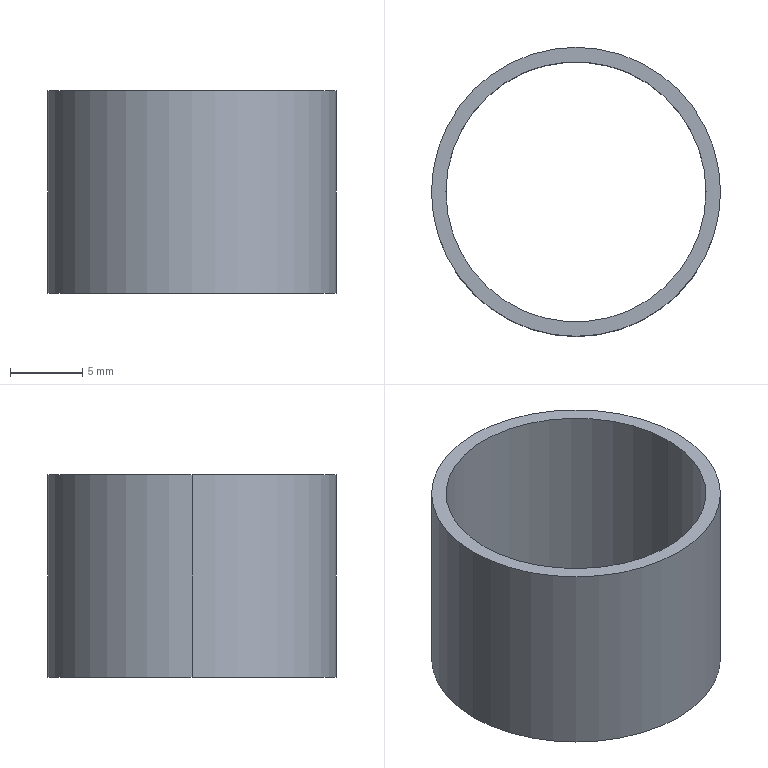Part | STEP file | Oil-Free Bushing JH-B-18-14 | 1 solid | 6 faces | box 20 x 20 x 14 mm | volume 835.664 mm3 | cylinder 4 | plane 2 | commonest cylinder face diameters 18 x2 20 x2
STEP:
#1=CARTESIAN_POINT('',(0.,0.,0.));
#2=DIRECTION('',(0.,0.,1.));
#3=DIRECTION('',(1.,0.,0.));
#4=AXIS2_PLACEMENT_3D('',#1,#2,#3);
#5=CARTESIAN_POINT('',(-9.,0.,14.));
#6=VERTEX_POINT('',#5);
#7=CARTESIAN_POINT('',(-9.,0.,0.));
#8=VERTEX_POINT('',#7);
#9=CARTESIAN_POINT('',(-9.,0.,14.));
#10=DIRECTION('',(0.,0.,-1.));
#11=VECTOR('',#10,1.);
#12=LINE('',#9,#11);
#13=CARTESIAN_POINT('',(0.,0.,14.));
#14=DIRECTION('',(0.,0.,-1.));
#15=DIRECTION('',(-1.,0.,0.));
#16=AXIS2_PLACEMENT_3D('',#13,#14,#15);
#17=CYLINDRICAL_SURFACE('',#16,9.);
#18=CARTESIAN_POINT('',(6.283,0.));
#19=DIRECTION('',(0.,1.));
#20=VECTOR('',#19,1.);
#21=LINE('',#18,#20);
#22=(GEOMETRIC_REPRESENTATION_CONTEXT(2)PARAMETRIC_REPRESENTATION_CONTEXT()REPRESENTATION_CONTEXT('',''));
#23=DEFINITIONAL_REPRESENTATION('',(#21),#22);
#24=PCURVE('',#17,#23);
#25=CARTESIAN_POINT('',(0.,0.,14.));
#26=DIRECTION('',(0.,0.,-1.));
#27=DIRECTION('',(-1.,0.,0.));
#28=AXIS2_PLACEMENT_3D('',#25,#26,#27);
#29=CYLINDRICAL_SURFACE('',#28,9.);
#30=CARTESIAN_POINT('',(0.,0.));
#31=DIRECTION('',(0.,1.));
#32=VECTOR('',#31,1.);
#33=LINE('',#30,#32);
#34=(GEOMETRIC_REPRESENTATION_CONTEXT(2)PARAMETRIC_REPRESENTATION_CONTEXT()REPRESENTATION_CONTEXT('',''));
#35=DEFINITIONAL_REPRESENTATION('',(#33),#34);
#36=PCURVE('',#29,#35);
#37=SURFACE_CURVE('',#12,(#24,#36),.PCURVE_S1.);
#38=EDGE_CURVE('',#6,#8,#37,.T.);
#39=ORIENTED_EDGE('',*,*,#38,.T.);
#40=CARTESIAN_POINT('',(9.,0.,0.));
#41=VERTEX_POINT('',#40);
#42=CARTESIAN_POINT('',(0.,0.,0.));
#43=DIRECTION('',(0.,0.,1.));
#44=DIRECTION('',(1.,0.,0.));
#45=AXIS2_PLACEMENT_3D('',#42,#43,#44);
#46=CIRCLE('',#45,9.);
#47=CARTESIAN_POINT('',(9.425,14.));
#48=DIRECTION('',(-1.,0.));
#49=VECTOR('',#48,1.);
#50=LINE('',#47,#49);
#51=(GEOMETRIC_REPRESENTATION_CONTEXT(2)PARAMETRIC_REPRESENTATION_CONTEXT()REPRESENTATION_CONTEXT('',''));
#52=DEFINITIONAL_REPRESENTATION('',(#50),#51);
#53=PCURVE('',#17,#52);
#54=CARTESIAN_POINT('',(0.,0.,0.));
#55=DIRECTION('',(0.,0.,1.));
#56=DIRECTION('',(1.,0.,0.));
#57=AXIS2_PLACEMENT_3D('',#54,#55,#56);
#58=PLANE('',#57);
#59=CARTESIAN_POINT('',(0.,0.));
#60=DIRECTION('',(1.,0.));
#61=AXIS2_PLACEMENT_2D('',#59,#60);
#62=CIRCLE('',#61,9.);
#63=(GEOMETRIC_REPRESENTATION_CONTEXT(2)PARAMETRIC_REPRESENTATION_CONTEXT()REPRESENTATION_CONTEXT('',''));
#64=DEFINITIONAL_REPRESENTATION('',(#62),#63);
#65=PCURVE('',#58,#64);
#66=SURFACE_CURVE('',#46,(#53,#65),.PCURVE_S1.);
#67=EDGE_CURVE('',#8,#41,#66,.T.);
#68=ORIENTED_EDGE('',*,*,#67,.T.);
#69=CARTESIAN_POINT('',(9.,0.,14.));
#70=VERTEX_POINT('',#69);
#71=CARTESIAN_POINT('',(9.,0.,14.));
#72=DIRECTION('',(0.,0.,-1.));
#73=VECTOR('',#72,1.);
#74=LINE('',#71,#73);
#75=CARTESIAN_POINT('',(3.142,0.));
#76=DIRECTION('',(0.,1.));
#77=VECTOR('',#76,1.);
#78=LINE('',#75,#77);
#79=(GEOMETRIC_REPRESENTATION_CONTEXT(2)PARAMETRIC_REPRESENTATION_CONTEXT()REPRESENTATION_CONTEXT('',''));
#80=DEFINITIONAL_REPRESENTATION('',(#78),#79);
#81=PCURVE('',#17,#80);
#82=CARTESIAN_POINT('',(3.142,0.));
#83=DIRECTION('',(0.,1.));
#84=VECTOR('',#83,1.);
#85=LINE('',#82,#84);
#86=(GEOMETRIC_REPRESENTATION_CONTEXT(2)PARAMETRIC_REPRESENTATION_CONTEXT()REPRESENTATION_CONTEXT('',''));
#87=DEFINITIONAL_REPRESENTATION('',(#85),#86);
#88=PCURVE('',#29,#87);
#89=SURFACE_CURVE('',#74,(#81,#88),.PCURVE_S1.);
#90=EDGE_CURVE('',#70,#41,#89,.T.);
#91=ORIENTED_EDGE('',*,*,#90,.F.);
#92=CARTESIAN_POINT('',(0.,0.,14.));
#93=DIRECTION('',(0.,0.,1.));
#94=DIRECTION('',(1.,0.,0.));
#95=AXIS2_PLACEMENT_3D('',#92,#93,#94);
#96=CIRCLE('',#95,9.);
#97=CARTESIAN_POINT('',(9.425,0.));
#98=DIRECTION('',(-1.,0.));
#99=VECTOR('',#98,1.);
#100=LINE('',#97,#99);
#101=(GEOMETRIC_REPRESENTATION_CONTEXT(2)PARAMETRIC_REPRESENTATION_CONTEXT()REPRESENTATION_CONTEXT('',''));
#102=DEFINITIONAL_REPRESENTATION('',(#100),#101);
#103=PCURVE('',#17,#102);
#104=CARTESIAN_POINT('',(0.,0.,14.));
#105=DIRECTION('',(0.,0.,1.));
#106=DIRECTION('',(1.,0.,0.));
#107=AXIS2_PLACEMENT_3D('',#104,#105,#106);
#108=PLANE('',#107);
#109=CARTESIAN_POINT('',(0.,0.));
#110=DIRECTION('',(1.,0.));
#111=AXIS2_PLACEMENT_2D('',#109,#110);
#112=CIRCLE('',#111,9.);
#113=(GEOMETRIC_REPRESENTATION_CONTEXT(2)PARAMETRIC_REPRESENTATION_CONTEXT()REPRESENTATION_CONTEXT('',''));
#114=DEFINITIONAL_REPRESENTATION('',(#112),#113);
#115=PCURVE('',#108,#114);
#116=SURFACE_CURVE('',#96,(#103,#115),.PCURVE_S1.);
#117=EDGE_CURVE('',#6,#70,#116,.T.);
#118=ORIENTED_EDGE('',*,*,#117,.F.);
#119=EDGE_LOOP('',(#39,#68,#91,#118));
#120=FACE_BOUND('',#119,.F.);
#121=ADVANCED_FACE('',(#120),#17,.F.);
#122=CARTESIAN_POINT('',(10.,0.,14.));
#123=VERTEX_POINT('',#122);
#124=CARTESIAN_POINT('',(-10.,0.,14.));
#125=VERTEX_POINT('',#124);
#126=CARTESIAN_POINT('',(0.,0.,14.));
#127=DIRECTION('',(0.,0.,1.));
#128=DIRECTION('',(1.,0.,0.));
#129=AXIS2_PLACEMENT_3D('',#126,#127,#128);
#130=CIRCLE('',#129,10.);
#131=CARTESIAN_POINT('',(0.,0.,14.));
#132=DIRECTION('',(0.,0.,-1.));
#133=DIRECTION('',(-1.,0.,0.));
#134=AXIS2_PLACEMENT_3D('',#131,#132,#133);
#135=CYLINDRICAL_SURFACE('',#134,10.);
#136=CARTESIAN_POINT('',(3.142,0.));
#137=DIRECTION('',(-1.,0.));
#138=VECTOR('',#137,1.);
#139=LINE('',#136,#138);
#140=(GEOMETRIC_REPRESENTATION_CONTEXT(2)PARAMETRIC_REPRESENTATION_CONTEXT()REPRESENTATION_CONTEXT('',''));
#141=DEFINITIONAL_REPRESENTATION('',(#139),#140);
#142=PCURVE('',#135,#141);
#143=CARTESIAN_POINT('',(0.,0.));
#144=DIRECTION('',(1.,0.));
#145=AXIS2_PLACEMENT_2D('',#143,#144);
#146=CIRCLE('',#145,10.);
#147=(GEOMETRIC_REPRESENTATION_CONTEXT(2)PARAMETRIC_REPRESENTATION_CONTEXT()REPRESENTATION_CONTEXT('',''));
#148=DEFINITIONAL_REPRESENTATION('',(#146),#147);
#149=PCURVE('',#108,#148);
#150=SURFACE_CURVE('',#130,(#142,#149),.PCURVE_S1.);
#151=EDGE_CURVE('',#123,#125,#150,.T.);
#152=ORIENTED_EDGE('',*,*,#151,.F.);
#153=CARTESIAN_POINT('',(10.,0.,0.));
#154=VERTEX_POINT('',#153);
#155=CARTESIAN_POINT('',(10.,0.,14.));
#156=DIRECTION('',(0.,0.,-1.));
#157=VECTOR('',#156,1.);
#158=LINE('',#155,#157);
#159=CARTESIAN_POINT('',(3.142,0.));
#160=DIRECTION('',(0.,1.));
#161=VECTOR('',#160,1.);
#162=LINE('',#159,#161);
#163=(GEOMETRIC_REPRESENTATION_CONTEXT(2)PARAMETRIC_REPRESENTATION_CONTEXT()REPRESENTATION_CONTEXT('',''));
#164=DEFINITIONAL_REPRESENTATION('',(#162),#163);
#165=PCURVE('',#135,#164);
#166=CARTESIAN_POINT('',(0.,0.,14.));
#167=DIRECTION('',(0.,0.,-1.));
#168=DIRECTION('',(-1.,0.,0.));
#169=AXIS2_PLACEMENT_3D('',#166,#167,#168);
#170=CYLINDRICAL_SURFACE('',#169,10.);
#171=CARTESIAN_POINT('',(3.142,0.));
#172=DIRECTION('',(0.,1.));
#173=VECTOR('',#172,1.);
#174=LINE('',#171,#173);
#175=(GEOMETRIC_REPRESENTATION_CONTEXT(2)PARAMETRIC_REPRESENTATION_CONTEXT()REPRESENTATION_CONTEXT('',''));
#176=DEFINITIONAL_REPRESENTATION('',(#174),#175);
#177=PCURVE('',#170,#176);
#178=SURFACE_CURVE('',#158,(#165,#177),.PCURVE_S1.);
#179=EDGE_CURVE('',#123,#154,#178,.T.);
#180=ORIENTED_EDGE('',*,*,#179,.T.);
#181=CARTESIAN_POINT('',(-10.,0.,0.));
#182=VERTEX_POINT('',#181);
#183=CARTESIAN_POINT('',(0.,0.,0.));
#184=DIRECTION('',(0.,0.,1.));
#185=DIRECTION('',(1.,0.,0.));
#186=AXIS2_PLACEMENT_3D('',#183,#184,#185);
#187=CIRCLE('',#186,10.);
#188=CARTESIAN_POINT('',(3.142,14.));
#189=DIRECTION('',(-1.,0.));
#190=VECTOR('',#189,1.);
#191=LINE('',#188,#190);
#192=(GEOMETRIC_REPRESENTATION_CONTEXT(2)PARAMETRIC_REPRESENTATION_CONTEXT()REPRESENTATION_CONTEXT('',''));
#193=DEFINITIONAL_REPRESENTATION('',(#191),#192);
#194=PCURVE('',#135,#193);
#195=CARTESIAN_POINT('',(0.,0.));
#196=DIRECTION('',(1.,0.));
#197=AXIS2_PLACEMENT_2D('',#195,#196);
#198=CIRCLE('',#197,10.);
#199=(GEOMETRIC_REPRESENTATION_CONTEXT(2)PARAMETRIC_REPRESENTATION_CONTEXT()REPRESENTATION_CONTEXT('',''));
#200=DEFINITIONAL_REPRESENTATION('',(#198),#199);
#201=PCURVE('',#58,#200);
#202=SURFACE_CURVE('',#187,(#194,#201),.PCURVE_S1.);
#203=EDGE_CURVE('',#154,#182,#202,.T.);
#204=ORIENTED_EDGE('',*,*,#203,.T.);
#205=CARTESIAN_POINT('',(-10.,0.,14.));
#206=DIRECTION('',(0.,0.,-1.));
#207=VECTOR('',#206,1.);
#208=LINE('',#205,#207);
#209=CARTESIAN_POINT('',(0.,0.));
#210=DIRECTION('',(0.,1.));
#211=VECTOR('',#210,1.);
#212=LINE('',#209,#211);
#213=(GEOMETRIC_REPRESENTATION_CONTEXT(2)PARAMETRIC_REPRESENTATION_CONTEXT()REPRESENTATION_CONTEXT('',''));
#214=DEFINITIONAL_REPRESENTATION('',(#212),#213);
#215=PCURVE('',#135,#214);
#216=CARTESIAN_POINT('',(6.283,0.));
#217=DIRECTION('',(0.,1.));
#218=VECTOR('',#217,1.);
#219=LINE('',#216,#218);
#220=(GEOMETRIC_REPRESENTATION_CONTEXT(2)PARAMETRIC_REPRESENTATION_CONTEXT()REPRESENTATION_CONTEXT('',''));
#221=DEFINITIONAL_REPRESENTATION('',(#219),#220);
#222=PCURVE('',#170,#221);
#223=SURFACE_CURVE('',#208,(#215,#222),.PCURVE_S1.);
#224=EDGE_CURVE('',#125,#182,#223,.T.);
#225=ORIENTED_EDGE('',*,*,#224,.F.);
#226=EDGE_LOOP('',(#152,#180,#204,#225));
#227=FACE_BOUND('',#226,.T.);
#228=ADVANCED_FACE('',(#227),#135,.T.);
#229=CARTESIAN_POINT('',(0.,0.,14.));
#230=DIRECTION('',(0.,0.,1.));
#231=DIRECTION('',(1.,0.,0.));
#232=AXIS2_PLACEMENT_3D('',#229,#230,#231);
#233=CIRCLE('',#232,10.);
#234=CARTESIAN_POINT('',(0.,0.));
#235=DIRECTION('',(1.,0.));
#236=AXIS2_PLACEMENT_2D('',#234,#235);
#237=CIRCLE('',#236,10.);
#238=(GEOMETRIC_REPRESENTATION_CONTEXT(2)PARAMETRIC_REPRESENTATION_CONTEXT()REPRESENTATION_CONTEXT('',''));
#239=DEFINITIONAL_REPRESENTATION('',(#237),#238);
#240=PCURVE('',#108,#239);
#241=CARTESIAN_POINT('',(9.425,0.));
#242=DIRECTION('',(-1.,0.));
#243=VECTOR('',#242,1.);
#244=LINE('',#241,#243);
#245=(GEOMETRIC_REPRESENTATION_CONTEXT(2)PARAMETRIC_REPRESENTATION_CONTEXT()REPRESENTATION_CONTEXT('',''));
#246=DEFINITIONAL_REPRESENTATION('',(#244),#245);
#247=PCURVE('',#170,#246);
#248=SURFACE_CURVE('',#233,(#240,#247),.PCURVE_S1.);
#249=EDGE_CURVE('',#125,#123,#248,.T.);
#250=ORIENTED_EDGE('',*,*,#249,.T.);
#251=ORIENTED_EDGE('',*,*,#151,.T.);
#252=EDGE_LOOP('',(#250,#251));
#253=FACE_BOUND('',#252,.T.);
#254=ORIENTED_EDGE('',*,*,#117,.F.);
#255=CARTESIAN_POINT('',(0.,0.,14.));
#256=DIRECTION('',(0.,0.,1.));
#257=DIRECTION('',(1.,0.,0.));
#258=AXIS2_PLACEMENT_3D('',#255,#256,#257);
#259=CIRCLE('',#258,9.);
#260=CARTESIAN_POINT('',(0.,0.));
#261=DIRECTION('',(1.,0.));
#262=AXIS2_PLACEMENT_2D('',#260,#261);
#263=CIRCLE('',#262,9.);
#264=(GEOMETRIC_REPRESENTATION_CONTEXT(2)PARAMETRIC_REPRESENTATION_CONTEXT()REPRESENTATION_CONTEXT('',''));
#265=DEFINITIONAL_REPRESENTATION('',(#263),#264);
#266=PCURVE('',#108,#265);
#267=CARTESIAN_POINT('',(3.142,0.));
#268=DIRECTION('',(-1.,0.));
#269=VECTOR('',#268,1.);
#270=LINE('',#267,#269);
#271=(GEOMETRIC_REPRESENTATION_CONTEXT(2)PARAMETRIC_REPRESENTATION_CONTEXT()REPRESENTATION_CONTEXT('',''));
#272=DEFINITIONAL_REPRESENTATION('',(#270),#271);
#273=PCURVE('',#29,#272);
#274=SURFACE_CURVE('',#259,(#266,#273),.PCURVE_S1.);
#275=EDGE_CURVE('',#70,#6,#274,.T.);
#276=ORIENTED_EDGE('',*,*,#275,.F.);
#277=EDGE_LOOP('',(#254,#276));
#278=FACE_BOUND('',#277,.T.);
#279=ADVANCED_FACE('',(#253,#278),#108,.T.);
#280=CARTESIAN_POINT('',(0.,0.,0.));
#281=DIRECTION('',(0.,0.,1.));
#282=DIRECTION('',(1.,0.,0.));
#283=AXIS2_PLACEMENT_3D('',#280,#281,#282);
#284=CIRCLE('',#283,10.);
#285=CARTESIAN_POINT('',(0.,0.));
#286=DIRECTION('',(1.,0.));
#287=AXIS2_PLACEMENT_2D('',#285,#286);
#288=CIRCLE('',#287,10.);
#289=(GEOMETRIC_REPRESENTATION_CONTEXT(2)PARAMETRIC_REPRESENTATION_CONTEXT()REPRESENTATION_CONTEXT('',''));
#290=DEFINITIONAL_REPRESENTATION('',(#288),#289);
#291=PCURVE('',#58,#290);
#292=CARTESIAN_POINT('',(9.425,14.));
#293=DIRECTION('',(-1.,0.));
#294=VECTOR('',#293,1.);
#295=LINE('',#292,#294);
#296=(GEOMETRIC_REPRESENTATION_CONTEXT(2)PARAMETRIC_REPRESENTATION_CONTEXT()REPRESENTATION_CONTEXT('',''));
#297=DEFINITIONAL_REPRESENTATION('',(#295),#296);
#298=PCURVE('',#170,#297);
#299=SURFACE_CURVE('',#284,(#291,#298),.PCURVE_S1.);
#300=EDGE_CURVE('',#182,#154,#299,.T.);
#301=ORIENTED_EDGE('',*,*,#300,.F.);
#302=ORIENTED_EDGE('',*,*,#203,.F.);
#303=EDGE_LOOP('',(#301,#302));
#304=FACE_BOUND('',#303,.T.);
#305=ORIENTED_EDGE('',*,*,#67,.T.);
#306=CARTESIAN_POINT('',(0.,0.,0.));
#307=DIRECTION('',(0.,0.,1.));
#308=DIRECTION('',(1.,0.,0.));
#309=AXIS2_PLACEMENT_3D('',#306,#307,#308);
#310=CIRCLE('',#309,9.);
#311=CARTESIAN_POINT('',(0.,0.));
#312=DIRECTION('',(1.,0.));
#313=AXIS2_PLACEMENT_2D('',#311,#312);
#314=CIRCLE('',#313,9.);
#315=(GEOMETRIC_REPRESENTATION_CONTEXT(2)PARAMETRIC_REPRESENTATION_CONTEXT()REPRESENTATION_CONTEXT('',''));
#316=DEFINITIONAL_REPRESENTATION('',(#314),#315);
#317=PCURVE('',#58,#316);
#318=CARTESIAN_POINT('',(3.142,14.));
#319=DIRECTION('',(-1.,0.));
#320=VECTOR('',#319,1.);
#321=LINE('',#318,#320);
#322=(GEOMETRIC_REPRESENTATION_CONTEXT(2)PARAMETRIC_REPRESENTATION_CONTEXT()REPRESENTATION_CONTEXT('',''));
#323=DEFINITIONAL_REPRESENTATION('',(#321),#322);
#324=PCURVE('',#29,#323);
#325=SURFACE_CURVE('',#310,(#317,#324),.PCURVE_S1.);
#326=EDGE_CURVE('',#41,#8,#325,.T.);
#327=ORIENTED_EDGE('',*,*,#326,.T.);
#328=EDGE_LOOP('',(#305,#327));
#329=FACE_BOUND('',#328,.T.);
#330=ADVANCED_FACE('',(#304,#329),#58,.F.);
#331=ORIENTED_EDGE('',*,*,#179,.F.);
#332=ORIENTED_EDGE('',*,*,#249,.F.);
#333=ORIENTED_EDGE('',*,*,#224,.T.);
#334=ORIENTED_EDGE('',*,*,#300,.T.);
#335=EDGE_LOOP('',(#331,#332,#333,#334));
#336=FACE_BOUND('',#335,.T.);
#337=ADVANCED_FACE('',(#336),#170,.T.);
#338=ORIENTED_EDGE('',*,*,#326,.T.);
#339=ORIENTED_EDGE('',*,*,#38,.F.);
#340=ORIENTED_EDGE('',*,*,#275,.F.);
#341=ORIENTED_EDGE('',*,*,#90,.T.);
#342=EDGE_LOOP('',(#338,#339,#340,#341));
#343=FACE_BOUND('',#342,.F.);
#344=ADVANCED_FACE('',(#343),#29,.F.);
#345=CLOSED_SHELL('',(#121,#228,#279,#330,#337,#344));
#346=MANIFOLD_SOLID_BREP('',#345);
#347=(LENGTH_UNIT()NAMED_UNIT(*)SI_UNIT(.MILLI.,.METRE.));
#348=UNCERTAINTY_MEASURE_WITH_UNIT(LENGTH_MEASURE(0.0000001),#347,'','');
#349=(NAMED_UNIT(*)PLANE_ANGLE_UNIT()SI_UNIT($,.RADIAN.));
#350=(NAMED_UNIT(*)SI_UNIT($,.STERADIAN.)SOLID_ANGLE_UNIT());
#351=(GEOMETRIC_REPRESENTATION_CONTEXT(3)GLOBAL_UNCERTAINTY_ASSIGNED_CONTEXT((#348))GLOBAL_UNIT_ASSIGNED_CONTEXT((#347,#349,#350))REPRESENTATION_CONTEXT('',''));
#352=ADVANCED_BREP_SHAPE_REPRESENTATION('',(#4,#346),#351);